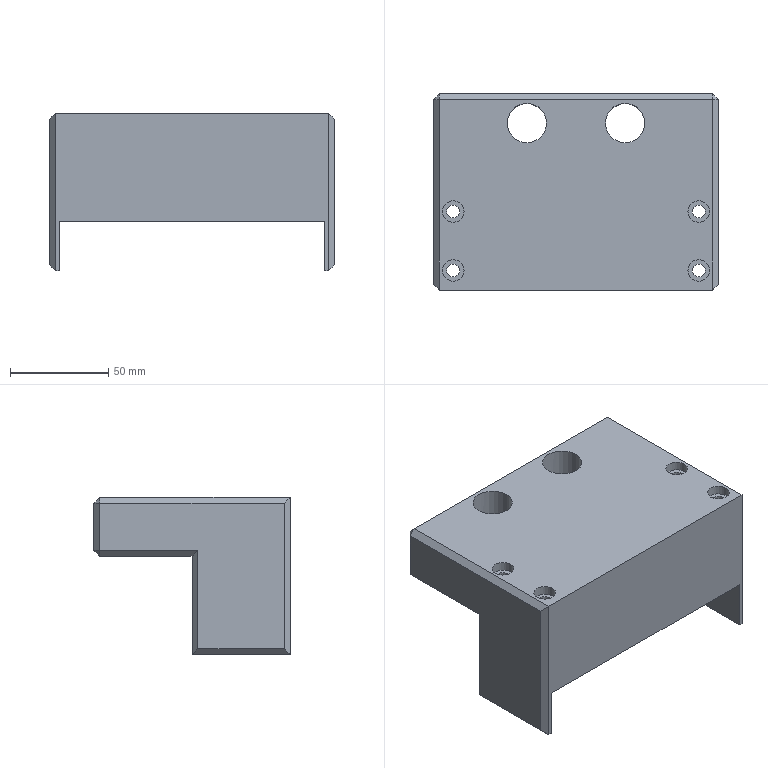NC program | NX | posted with a generic post | part box 145 x 100 x 80 mm
Whole program:
N10 G17 G21 G94 G90
(FLOOR_WALL_2_COPY , TOOL : D63)
N12 T01 M6
N14 G54
N16 G17 G0 G90 X38.997 Y86.956 B0. C0. S6500 M3
N18 G43 Z30. H1
N20 Z0.504
N22 G94 G1 Z-0.996 F1000.
N24 G3 X35.847 Y81.5 R6.3
N26 G1 Y-31.5 F1500.
N28 X-0.001
N30 Y81.5
N32 X-35.85
N34 Y-31.5
N36 G3 X-32.7 Y-36.956 R6.3
N38 G1 Z0.504
N40 G0 Z30.
N42 X38.997 Y86.956
N44 Z-0.492
N46 G1 Z-1.992 F1000.
N48 G3 X35.847 Y81.5 R6.3
N50 G1 Y-31.5 F1500.
N52 X-0.001
N54 Y81.5
N56 X-35.85
N58 Y-31.5
N60 G3 X-32.7 Y-36.956 R6.3
N62 G1 Z-0.492
N64 G0 Z30.
N66 X38.997 Y86.956
N68 Z-1.488
N70 G1 Z-2.988 F1000.
N72 G3 X35.847 Y81.5 R6.3
N74 G1 Y-31.5 F1500.
N76 X-0.001
N78 Y81.5
N80 X-35.85
N82 Y-31.5
N84 G3 X-32.7 Y-36.956 R6.3
N86 G1 Z-1.488
N88 G0 Z30.
N90 X38.997 Y86.956
N92 Z-2.484
N94 G1 Z-3.984 F1000.
N96 G3 X35.847 Y81.5 R6.3
N98 G1 Y-31.5 F1500.
N100 X-0.001
N102 Y81.5
N104 X-35.85
N106 Y-31.5
N108 G3 X-32.7 Y-36.956 R6.3
N110 G1 Z-2.484
N112 G0 Z30.
N114 X38.997 Y86.956
N116 Z-3.48
N118 G1 Z-4.98 F1000.
N120 G3 X35.847 Y81.5 R6.3
N122 G1 Y-31.5 F1500.
N124 X-0.001
N126 Y81.5
N128 X-35.85
N130 Y-31.5
N132 G3 X-32.7 Y-36.956 R6.3
N134 G1 Z-3.48
N136 G0 Z30.
N138 X38.997 Y86.956
N140 Z-4.476
N142 G1 Z-5.976 F1000.
N144 G3 X35.847 Y81.5 R6.3
N146 G1 Y-31.5 F1500.
N148 X-0.001
N150 Y81.5
N152 X-35.85
N154 Y-31.5
N156 G3 X-32.7 Y-36.956 R6.3
N158 G1 Z-4.476
N160 G0 Z30.
N162 X38.997 Y86.956
N164 Z-5.472
N166 G1 Z-6.972 F1000.
N168 G3 X35.847 Y81.5 R6.3
N170 G1 Y-31.5 F1500.
N172 X-0.001
N174 Y81.5
N176 X-35.85
N178 Y-31.5
N180 G3 X-32.7 Y-36.956 R6.3
N182 G1 Z-5.472
N184 G0 Z30.
N186 X38.997 Y86.956
N188 Z-6.468
N190 G1 Z-7.968 F1000.
N192 G3 X35.847 Y81.5 R6.3
N194 G1 Y-31.5 F1500.
N196 X-0.001
N198 Y81.5
N200 X-35.85
N202 Y-31.5
N204 G3 X-32.7 Y-36.956 R6.3
N206 G1 Z-6.468
N208 G0 Z30.
N210 X38.997 Y86.956
N212 Z-7.464
N214 G1 Z-8.964 F1000.
N216 G3 X35.847 Y81.5 R6.3
N218 G1 Y-31.5 F1500.
N220 X-0.001
N222 Y81.5
N224 X-35.85
N226 Y-31.5
N228 G3 X-32.7 Y-36.956 R6.3
N230 G1 Z-7.464
N232 G0 Z30.
N234 X38.997 Y86.956
N236 Z-8.46
N238 G1 Z-9.96 F1000.
N240 G3 X35.847 Y81.5 R6.3
N242 G1 Y-31.5 F1500.
N244 X-0.001
N246 Y81.5
N248 X-35.85
N250 Y-31.5
N252 G3 X-32.7 Y-36.956 R6.3
N254 G1 Z-8.46
N256 G0 Z30.
N258 X38.997 Y86.956
N260 Z-9.456
N262 G1 Z-10.956 F1000.
N264 G3 X35.847 Y81.5 R6.3
N266 G1 Y-31.5 F1500.
N268 X-0.001
N270 Y81.5
N272 X-35.85
N274 Y-31.5
N276 G3 X-32.7 Y-36.956 R6.3
N278 G1 Z-9.456
N280 G0 Z30.
N282 X38.997 Y86.956
N284 Z-10.452
N286 G1 Z-11.952 F1000.
N288 G3 X35.847 Y81.5 R6.3
N290 G1 Y-31.5 F1500.
N292 X-0.001
N294 Y81.5
N296 X-35.85
N298 Y-31.5
N300 G3 X-32.7 Y-36.956 R6.3
N302 G1 Z-10.452
N304 G0 Z30.
N306 X38.997 Y86.956
N308 Z-11.448
N310 G1 Z-12.948 F1000.
N312 G3 X35.847 Y81.5 R6.3
N314 G1 Y-31.5 F1500.
N316 X-0.001
N318 Y81.5
N320 X-35.85
N322 Y-31.5
N324 G3 X-32.7 Y-36.956 R6.3
N326 G1 Z-11.448
N328 G0 Z30.
N330 X38.997 Y86.956
N332 Z-12.444
N334 G1 Z-13.944 F1000.
N336 G3 X35.847 Y81.5 R6.3
N338 G1 Y-31.5 F1500.
N340 X-0.001
N342 Y81.5
N344 X-35.85
N346 Y-31.5
N348 G3 X-32.7 Y-36.956 R6.3
N350 G1 Z-12.444
N352 G0 Z30.
N354 X38.997 Y86.956
N356 Z-13.44
N358 G1 Z-14.94 F1000.
N360 G3 X35.847 Y81.5 R6.3
N362 G1 Y-31.5 F1500.
N364 X-0.001
N366 Y81.5
N368 X-35.85
N370 Y-31.5
N372 G3 X-32.7 Y-36.956 R6.3
N374 G1 Z-13.44
N376 G0 Z30.
N378 X38.997 Y86.956
N380 Z-14.436
N382 G1 Z-15.936 F1000.
N384 G3 X35.847 Y81.5 R6.3
N386 G1 Y-31.5 F1500.
N388 X-0.001
N390 Y81.5
N392 X-35.85
N394 Y-31.5
N396 G3 X-32.7 Y-36.956 R6.3
N398 G1 Z-14.436
N400 G0 Z30.
N402 X38.997 Y86.956
N404 Z-15.432
N406 G1 Z-16.932 F1000.
N408 G3 X35.847 Y81.5 R6.3
N410 G1 Y-31.5 F1500.
N412 X-0.001
N414 Y81.5
N416 X-35.85
N418 Y-31.5
N420 G3 X-32.7 Y-36.956 R6.3
N422 G1 Z-15.432
N424 G0 Z30.
N426 X38.997 Y86.956
N428 Z-16.428
N430 G1 Z-17.928 F1000.
N432 G3 X35.847 Y81.5 R6.3
N434 G1 Y-31.5 F1500.
N436 X-0.001
N438 Y81.5
N440 X-35.85
N442 Y-31.5
N444 G3 X-32.7 Y-36.956 R6.3
N446 G1 Z-16.428
N448 G0 Z30.
N450 X38.997 Y86.956
N452 Z-17.424
N454 G1 Z-18.924 F1000.
N456 G3 X35.847 Y81.5 R6.3
N458 G1 Y-31.5 F1500.
N460 X-0.001
N462 Y81.5
N464 X-35.85
N466 Y-31.5
N468 G3 X-32.7 Y-36.956 R6.3
N470 G1 Z-17.424
N472 G0 Z30.
N474 X38.997 Y86.956
N476 Z-18.42
N478 G1 Z-19.92 F1000.
N480 G3 X35.847 Y81.5 R6.3
N482 G1 Y-31.5 F1500.
N484 X-0.001
N486 Y81.5
N488 X-35.85
N490 Y-31.5
N492 G3 X-32.7 Y-36.956 R6.3
N494 G1 Z-18.42
N496 G0 Z30.
N498 X38.997 Y86.956
N500 Z-19.416
N502 G1 Z-20.916 F1000.
N504 G3 X35.847 Y81.5 R6.3
N506 G1 Y-31.5 F1500.
N508 X-0.001
N510 Y81.5
N512 X-35.85
N514 Y-31.5
N516 G3 X-32.7 Y-36.956 R6.3
N518 G1 Z-19.416
N520 G0 Z30.
N522 X38.997 Y86.956
N524 Z-20.412
N526 G1 Z-21.912 F1000.
N528 G3 X35.847 Y81.5 R6.3
N530 G1 Y-31.5 F1500.
N532 X-0.001
N534 Y81.5
N536 X-35.85
N538 Y-31.5
N540 G3 X-32.7 Y-36.956 R6.3
N542 G1 Z-20.412
N544 G0 Z30.
N546 X38.997 Y86.956
N548 Z-21.408
N550 G1 Z-22.908 F1000.
N552 G3 X35.847 Y81.5 R6.3
N554 G1 Y-31.5 F1500.
N556 X-0.001
N558 Y81.5
N560 X-35.85
N562 Y-31.5
N564 G3 X-32.7 Y-36.956 R6.3
N566 G1 Z-21.408
N568 G0 Z30.
N570 X38.997 Y86.956
N572 Z-22.404
N574 G1 Z-23.904 F1000.
N576 G3 X35.847 Y81.5 R6.3
N578 G1 Y-31.5 F1500.
N580 X-0.001
N582 Y81.5
N584 X-35.85
N586 Y-31.5
N588 G3 X-32.7 Y-36.956 R6.3
N590 G1 Z-22.404
N592 G0 Z30.
N594 X38.997 Y86.956
N596 Z-23.4
N598 G1 Z-24.9 F1000.
N600 G3 X35.847 Y81.5 R6.3
N602 G1 Y-31.5 F1500.
N604 X-0.001
N606 Y81.5
N608 X-35.85
N610 Y-31.5
N612 G3 X-32.7 Y-36.956 R6.3
N614 G1 Z-23.4
N616 G0 Z30.
N618 M5
(FLOOR_WALL_1_COPY_COPY_COPY_COPY_COPY , TOOL : D10JING)
N620 T04 M6
N622 G54
N624 G17 G0 G90 X-61. Y56.443 B0. C0. S7500 M3
N626 G43 Z30. H4
N628 Z-10.95
N630 G94 G1 Z-12.45 F1250.
N632 X-62. Y55.866
N634 G3 X-62.5 Y55. R1.
N636 G1 Y-5.
N638 G3 X-62. Y-5.866 R1.
N640 G1 X-61. Y-6.443
N642 Z-10.95
N644 G0 Z30.
N646 X61.
N648 Z-10.95
N650 G1 Z-12.45
N652 X62. Y-5.866
N654 G3 X62.5 Y-5. R1.
N656 G1 Y55.
N658 G3 X62. Y55.866 R1.
N660 G1 X61. Y56.443
N662 Z-10.95
N664 G0 Z30.
N666 Y-6.443
N668 Z-23.4
N670 G1 Z-24.9
N672 X62. Y-5.866
N674 G3 X62.5 Y-5. R1.
N676 G1 Y55.
N678 G3 X62. Y55.866 R1.
N680 G1 X61. Y56.443
N682 Z-23.4
N684 G0 Z30.
N686 X-61.
N688 Z-23.4
N690 G1 Z-24.9
N692 X-62. Y55.866
N694 G3 X-62.5 Y55. R1.
N696 G1 Y-5.
N698 G3 X-62. Y-5.866 R1.
N700 G1 X-61. Y-6.443
N702 Z-23.4
N704 G0 Z30.
(FLOOR_WALL_1_COPY_COPY_COPY_COPY_1 , TOOL : D10JING)
N706 X61.499 Y56.5
N708 Z-23.5
N710 G1 Z-25.
N712 Y54.134
N714 G3 X61.999 Y55. R1.
N716 G1 Y-5.
N718 X57.039
N720 Y55.
N722 X52.079
N724 Y-5.
N726 X47.119
N728 Y55.
N730 X42.159
N732 Y-5.
N734 X37.199
N736 Y55.
N738 X32.239
N740 Y-5.
N742 X27.279
N744 Y55.
N746 X22.319
N748 Y-5.
N750 X17.359
N752 Y55.
N754 X12.399
N756 Y-5.
N758 X7.439
N760 Y55.
N762 X2.479
N764 Y-5.
N766 X-2.48
N768 Y55.
N770 X-7.44
N772 Y-5.
N774 X-12.4
N776 Y55.
N778 X-17.36
N780 Y-5.
N782 X-22.32
N784 Y55.
N786 X-27.28
N788 Y-5.
N790 X-32.24
N792 Y55.
N794 X-37.2
N796 Y-5.
N798 X-42.16
N800 Y55.
N802 X-47.12
N804 Y-5.
N806 X-52.08
N808 Y55.
N810 X-57.04
N812 Y-5.
N814 X-62.
N816 Y55.
N818 G2 X-61.5 Y55.866 R1.
N820 G1 X-60.402 Y56.5
N822 Z-23.5
N824 G0 Z30.
N826 X-60.902
N828 Z-23.5
N830 G1 Z-25.
N832 X-62. Y55.866
N834 G3 X-62.5 Y55. R1.
N836 G1 Y-5.
N838 G3 X-62. Y-5.866 R1.
N840 G1 X-60.902 Y-6.5
N842 Z-23.5
N844 G0 Z30.
N846 X60.902
N848 Z-23.5
N850 G1 Z-25.
N852 X62. Y-5.866
N854 G3 X62.5 Y-5. R1.
N856 G1 Y55.
N858 G3 X62. Y55.866 R1.
N860 G1 X60.902 Y56.5
N862 Z-23.5
N864 G0 Z30.
N866 M5
(ZLEVEL_PROFILE_1_COPY_1_COPY_COPY_1_COPY_COPY_COPY_COPY_COPY_1 , TOOL : D8A45)
N868 T06 M6
N870 G54
N872 G17 G0 G90 X-75.405 Y-1.526 B0. C0. S7500 M3
N874 G43 Z30. H6
N876 Z-2.5
N878 G94 G1 Z-3.5 F1000.
N880 X-74.386 Y-0.92
N882 G3 X-73.994 Y-0.223 R0.8
N884 G1 X-74. Y0.223
N886 Y47.002
N888 X-73.999 Y50.004
N890 G2 X-69.501 Y54.5 R4.498
N892 G1 X-67.499
N894 G2 X-63. Y50.001 R4.499
N896 G1 Y-0.001
N898 G2 X-67.499 Y-4.5 R4.504
N900 G1 X-69.501
N902 G2 X-73.994 Y-0.223 R4.505
N904 G3 X-74.429 Y0.449 R0.8
N906 G1 X-75.6 Y1.048
N908 Z-2.5
N910 G0 Z30.
N912 X75.457 Y51.309
N914 Z-2.5
N916 G1 Z-3.5
N918 X74.399 Y50.697
N920 G3 X73.999 Y50.004 R0.8
N922 G1 X74. Y47.002
N924 Y0.223
N926 X73.994 Y-0.223
N928 G2 X69.501 Y-4.5 R4.505
N930 G1 X67.499
N932 G2 X63. Y-0.001 R4.504
N934 G1 Y50.001
N936 G2 X67.499 Y54.5 R4.499
N938 G1 X69.501
N940 G2 X73.999 Y50.004 R4.498
N942 G3 X74.399 Y49.311 R0.8
N944 G1 X75.599 Y48.619
N946 Z-2.5
N948 G0 Z30.
(ZLEVEL_PROFILE_1_COPY_1_COPY_COPY_1_COPY_COPY_COPY_COPY_COPY_1_COPY , TOOL : D)
N950 X-74.377 Y-1.49
N952 Z-2.5
N954 G1 Z-3.5
N956 X-73.384 Y-0.898
N958 G3 X-72.994 Y-0.199 R0.8
N960 G1 X-73. Y0.199
N962 Y47.001
N964 Y50.017
N966 G2 X-69.501 Y53.5 R3.504
N968 G1 X-67.499
N970 G2 X-64. Y50.001 R3.499
N972 G1 Y-0.001
N974 G2 X-67.499 Y-3.5 R3.499
N976 G1 X-69.501
N978 G2 X-72.994 Y-0.199 R3.504
N980 G3 X-73.434 Y0.469 R0.8
N982 G1 X-74.6 Y1.055
N984 Z-2.5
N986 G0 Z30.
N988 X74.429 Y51.305
N990 Z-2.5
N992 G1 Z-3.5
N994 X73.4 Y50.71
N996 G3 X73. Y50.017 R0.8
N998 G1 Y47.001
N1000 Y0.199
N1002 X72.994 Y-0.199
N1004 G2 X69.501 Y-3.5 R3.504
N1006 G1 X67.499
N1008 G2 X64. Y-0.001 R3.499
N1010 G1 Y50.001
N1012 G2 X67.499 Y53.5 R3.499
N1014 G1 X69.501
N1016 G2 X73. Y50.017 R3.504
N1018 G3 X73.404 Y49.327 R0.8
N1020 G1 X74.6 Y48.646
N1022 Z-2.5
N1024 G0 Z30.
(ZLEVEL_PROFILE_1_COPY_1_COPY_COPY_1_COPY_COPY_COPY_COPY_COPY_1_COPY_COPY , TOO)
N1026 X62.1 Y40.673
N1028 Z-25.
N1030 G1 Z-26.
N1032 X63. Y41.514
N1034 G3 X63.4 Y42.207 R0.8
N1036 X63.395 Y37.792 R-2.383
N1038 X62.995 Y38.484 R0.8
N1040 G1 X62.1 Y39.327
N1042 Z-25.
N1044 G0 Z30.
N1046 Y10.673
N1048 Z-25.
N1050 G1 Z-26.
N1052 X62.997 Y11.515
N1054 G3 X63.397 Y12.208 R0.8
N1056 X63.393 Y7.791 R-2.383
N1058 X62.993 Y8.484 R0.8
N1060 G1 X62.1 Y9.327
N1062 Z-25.
N1064 G0 Z30.
N1066 X-62.1 Y39.327
N1068 Z-25.
N1070 G1 Z-26.
N1072 X-62.998 Y38.486
N1074 G3 X-63.398 Y37.793 R0.8
N1076 X-63.399 Y42.207 R-2.383
N1078 X-62.999 Y41.514 R0.8
N1080 G1 X-62.1 Y40.673
N1082 Z-25.
N1084 G0 Z30.
N1086 Y9.327
N1088 Z-25.
N1090 G1 Z-26.
N1092 X-63.002 Y8.487
N1094 G3 X-63.402 Y7.794 R0.8
N1096 X-63.399 Y12.207 R-2.383
N1098 X-62.999 Y11.514 R0.8
N1100 G1 X-62.1 Y10.673
N1102 Z-25.
N1104 G0 Z30.
N1106 X-62.432 Y52.517
N1108 Z-25.
N1110 G1 Z-26.
N1112 X-63.283 Y51.687
N1114 G3 X-63.499 Y50.917 R0.8
N1116 G1 X63.499
N1118 G3 X63.283 Y51.687 R0.8
N1120 G1 X62.432 Y52.517
N1122 Z-25.
N1124 G0 Z30.
N1126 X62.433 Y-2.517
N1128 Z-25.
N1130 G1 Z-26.
N1132 X63.283 Y-1.687
N1134 G3 X63.499 Y-0.917 R0.8
N1136 G1 X-63.499
N1138 G3 X-63.283 Y-1.687 R0.8
N1140 G1 X-62.433 Y-2.517
N1142 Z-25.
N1144 G0 Z30.
(ZLEVEL_PROFILE_1_COPY_1_COPY_COPY_1_COPY_COPY_COPY_COPY_COPY_1_COPY_COPY_COPY )
N1146 X23.53 Y-42.337
N1148 Z-50.
N1150 G1 Z-51.
N1152 X24.307 Y-43.683
N1154 G3 X25. Y-44.083 R0.8
N1156 X34.083 Y-35. R9.083
N1158 X25. Y-44.083 R-9.083
N1160 X25.693 Y-43.683 R0.8
N1162 G1 X26.47 Y-42.337
N1164 Z-50.
N1166 G0 Z30.
N1168 X-26.47
N1170 Z-50.
N1172 G1 Z-51.
N1174 X-25.693 Y-43.683
N1176 G3 X-25. Y-44.083 R0.8
N1178 X-15.917 Y-35. R9.083
N1180 X-25. Y-44.083 R-9.083
N1182 X-24.307 Y-43.683 R0.8
N1184 G1 X-23.53 Y-42.337
N1186 Z-50.
N1188 G0 Z30.
N1190 M5
N1192 M2